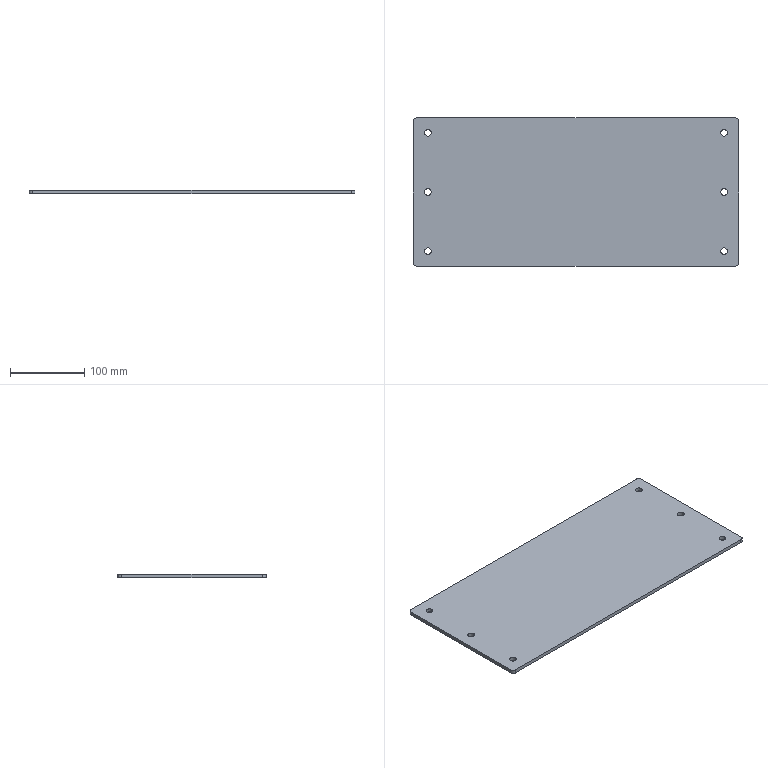Part | STEP file | 1 solid | 22 faces | box 440 x 200 x 5 mm | volume 437984 mm3 | cylinder 16 | plane 6 | commonest cylinder face diameters 9 x12 10 x4